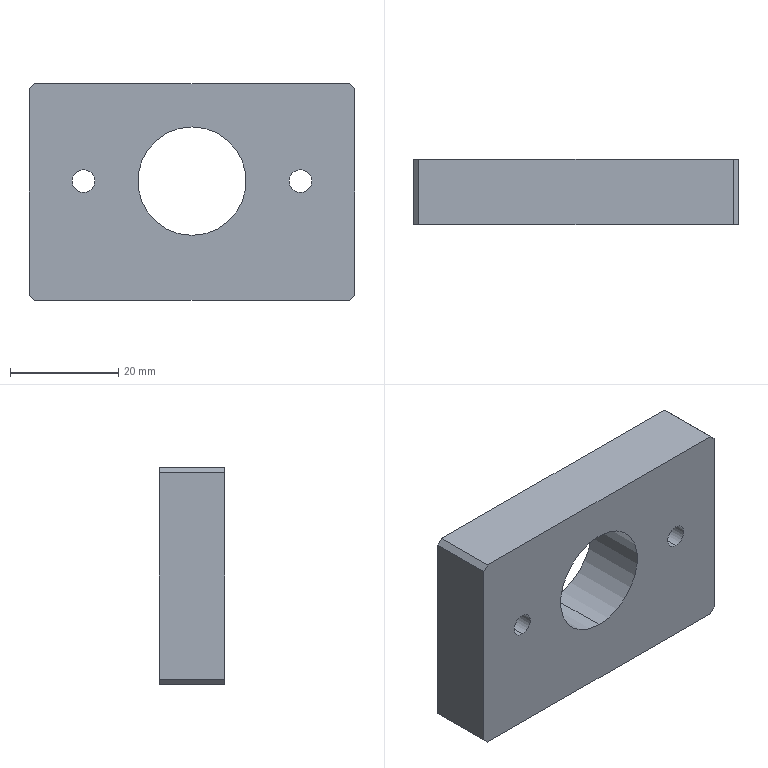Part | STEP file | 227H056249 Cylinder BKT_Default | 1 solid | 24 faces | box 60 x 12 x 40 mm | volume 24374 mm3 | cylinder 10 | plane 10 | cone 4 | commonest cylinder face diameters 4.2 x8 20 x2